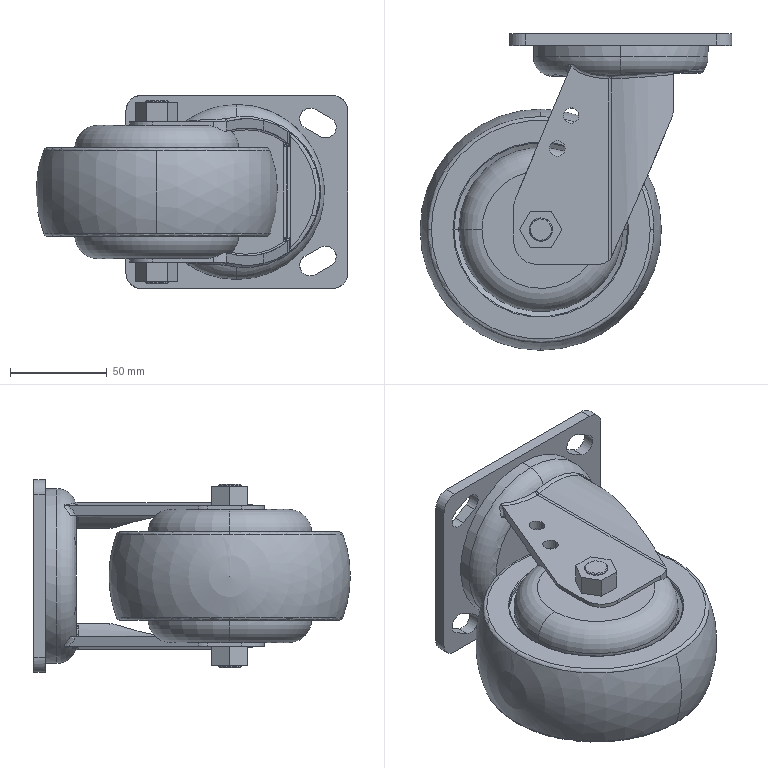Part | SolidWorks | features BaseBody 1 | 1 solid | 181 faces | box 161.5 x 164 x 100 mm | volume 842029 mm3 | plane 61 | cylinder 58 | torus 24 | spline 23 | cone 13 | sphere 2 | commonest cylinder face diameters 11 x12 8 x8 12 x4 16 x4 20 x4 24 x4